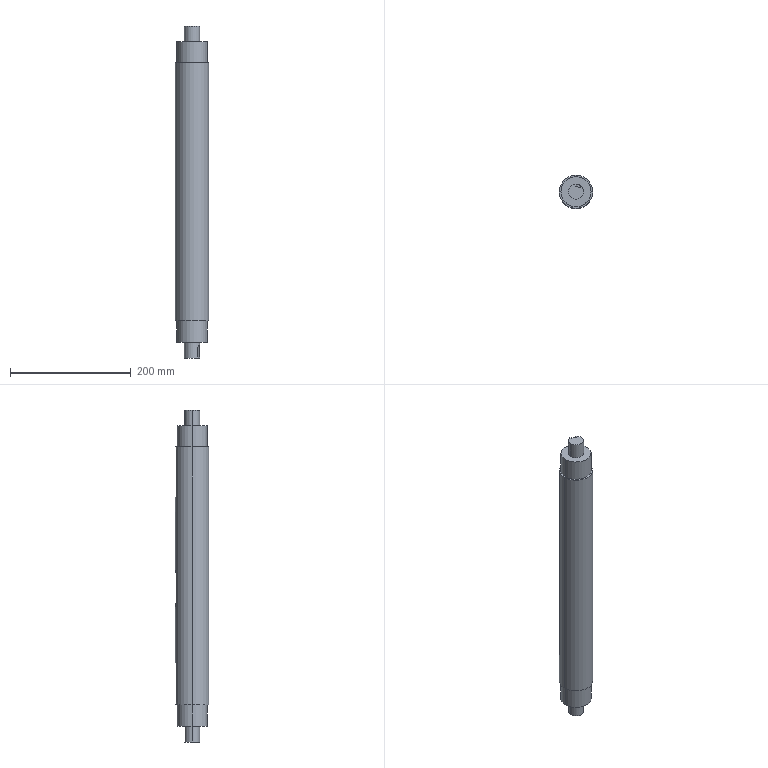Part | SolidWorks | features Cut 2, ICE 1, Revolution 1 | 1 solid | 30 faces | box 55 x 55 x 548.93 mm | volume 1170773 mm3 | cylinder 15 | plane 15 | commonest cylinder face diameters 25 x4 50 x4 16 x3 8 x2 55 x2
STEP:
#1=CARTESIAN_POINT('',(0.,21.5,183.93));
#2=VERTEX_POINT('',#1);
#3=CARTESIAN_POINT('',(8.,21.5,175.93));
#4=VERTEX_POINT('',#3);
#5=CARTESIAN_POINT('',(0.,21.5,175.93));
#6=DIRECTION('',(0.,1.,0.));
#7=DIRECTION('',(0.,0.,1.));
#8=AXIS2_PLACEMENT_3D('',#5,#6,#7);
#9=CIRCLE('',#8,8.);
#10=EDGE_CURVE('',#2,#4,#9,.T.);
#11=ORIENTED_EDGE('',*,*,#10,.F.);
#12=CARTESIAN_POINT('',(0.,27.5,183.93));
#13=VERTEX_POINT('',#12);
#14=CARTESIAN_POINT('',(0.,21.5,183.93));
#15=DIRECTION('',(0.,1.,0.));
#16=VECTOR('',#15,1000.);
#17=LINE('',#14,#16);
#18=EDGE_CURVE('',#2,#13,#17,.T.);
#19=ORIENTED_EDGE('',*,*,#18,.T.);
#20=CARTESIAN_POINT('',(8.,26.311,175.93));
#21=VERTEX_POINT('',#20);
#22=CARTESIAN_POINT('',(0.,27.5,183.93));
#23=CARTESIAN_POINT('',(0.5246,27.5,183.93));
#24=CARTESIAN_POINT('',(1.057,27.484,183.877));
#25=CARTESIAN_POINT('',(2.085,27.426,183.671));
#26=CARTESIAN_POINT('',(2.585,27.383,183.519));
#27=CARTESIAN_POINT('',(3.313,27.301,183.216));
#28=CARTESIAN_POINT('',(3.552,27.271,183.103));
#29=CARTESIAN_POINT('',(4.012,27.207,182.856));
#30=CARTESIAN_POINT('',(4.235,27.173,182.722));
#31=CARTESIAN_POINT('',(4.666,27.102,182.433));
#32=CARTESIAN_POINT('',(4.875,27.065,182.278));
#33=CARTESIAN_POINT('',(5.278,26.99,181.948));
#34=CARTESIAN_POINT('',(5.473,26.951,181.771));
#35=CARTESIAN_POINT('',(6.027,26.834,181.217));
#36=CARTESIAN_POINT('',(6.356,26.757,180.816));
#37=CARTESIAN_POINT('',(6.934,26.613,179.953));
#38=CARTESIAN_POINT('',(7.186,26.545,179.485));
#39=CARTESIAN_POINT('',(7.586,26.434,178.522));
#40=CARTESIAN_POINT('',(7.739,26.389,178.024));
#41=CARTESIAN_POINT('',(7.895,26.342,177.25));
#42=CARTESIAN_POINT('',(7.934,26.331,176.987));
#43=CARTESIAN_POINT('',(7.987,26.315,176.46));
#44=CARTESIAN_POINT('',(8.,26.311,176.196));
#45=CARTESIAN_POINT('',(8.,26.311,175.93));
#46=B_SPLINE_CURVE_WITH_KNOTS('',3,(#22,#23,#24,#25,#26,#27,#28,#29,#30,#31,#32,#33,#34,#35,#36,#37,#38,#39,#40,#41,#42,#43,#44,#45),.UNSPECIFIED.,.F.,.F.,(4,2,2,2,2,2,2,2,2,2,2,4),(0.01258,0.01415,0.01572,0.0165,0.01729,0.01807,0.01886,0.02043,0.022,0.02357,0.02435,0.02514),.UNSPECIFIED.);
#47=EDGE_CURVE('',#13,#21,#46,.T.);
#48=ORIENTED_EDGE('',*,*,#47,.T.);
#49=CARTESIAN_POINT('',(8.,21.5,175.93));
#50=DIRECTION('',(0.,1.,0.));
#51=VECTOR('',#50,1000.);
#52=LINE('',#49,#51);
#53=EDGE_CURVE('',#4,#21,#52,.T.);
#54=ORIENTED_EDGE('',*,*,#53,.F.);
#55=EDGE_LOOP('',(#11,#19,#48,#54));
#56=FACE_OUTER_BOUND('',#55,.T.);
#57=CARTESIAN_POINT('',(0.,21.5,175.93));
#58=DIRECTION('',(0.,1.,0.));
#59=DIRECTION('',(0.,0.,1.));
#60=AXIS2_PLACEMENT_3D('',#57,#58,#59);
#61=CYLINDRICAL_SURFACE('',#60,8.);
#62=ADVANCED_FACE('',(#56),#61,.F.);
#63=CARTESIAN_POINT('',(-25.,0.,422.93));
#64=VERTEX_POINT('',#63);
#65=CARTESIAN_POINT('',(25.,0.,422.93));
#66=VERTEX_POINT('',#65);
#67=CARTESIAN_POINT('',(0.,0.,422.93));
#68=DIRECTION('',(0.,0.,-1.));
#69=DIRECTION('',(-1.,0.,0.));
#70=AXIS2_PLACEMENT_3D('',#67,#68,#69);
#71=CIRCLE('',#70,25.);
#72=EDGE_CURVE('',#64,#66,#71,.T.);
#73=ORIENTED_EDGE('',*,*,#72,.T.);
#74=CARTESIAN_POINT('',(25.,0.,387.93));
#75=VERTEX_POINT('',#74);
#76=CARTESIAN_POINT('',(25.,0.,0.));
#77=DIRECTION('',(0.,0.,-1.));
#78=VECTOR('',#77,1000.);
#79=LINE('',#76,#78);
#80=EDGE_CURVE('',#66,#75,#79,.T.);
#81=ORIENTED_EDGE('',*,*,#80,.T.);
#82=CARTESIAN_POINT('',(-25.,0.,387.93));
#83=VERTEX_POINT('',#82);
#84=CARTESIAN_POINT('',(0.,0.,387.93));
#85=DIRECTION('',(0.,0.,-1.));
#86=DIRECTION('',(-1.,0.,0.));
#87=AXIS2_PLACEMENT_3D('',#84,#85,#86);
#88=CIRCLE('',#87,25.);
#89=EDGE_CURVE('',#83,#75,#88,.T.);
#90=ORIENTED_EDGE('',*,*,#89,.F.);
#91=CARTESIAN_POINT('',(-25.,0.,0.));
#92=DIRECTION('',(0.,0.,-1.));
#93=VECTOR('',#92,1000.);
#94=LINE('',#91,#93);
#95=EDGE_CURVE('',#64,#83,#94,.T.);
#96=ORIENTED_EDGE('',*,*,#95,.F.);
#97=EDGE_LOOP('',(#73,#81,#90,#96));
#98=FACE_OUTER_BOUND('',#97,.T.);
#99=CARTESIAN_POINT('',(0.,0.,0.));
#100=DIRECTION('',(0.,0.,-1.));
#101=DIRECTION('',(-1.,0.,0.));
#102=AXIS2_PLACEMENT_3D('',#99,#100,#101);
#103=CYLINDRICAL_SURFACE('',#102,25.);
#104=ADVANCED_FACE('',(#98),#103,.T.);
#105=CARTESIAN_POINT('',(-8.,26.311,175.93));
#106=VERTEX_POINT('',#105);
#107=CARTESIAN_POINT('',(-8.,26.311,175.93));
#108=CARTESIAN_POINT('',(-8.,26.311,176.462));
#109=CARTESIAN_POINT('',(-7.947,26.327,176.984));
#110=CARTESIAN_POINT('',(-7.794,26.373,177.754));
#111=CARTESIAN_POINT('',(-7.73,26.391,178.009));
#112=CARTESIAN_POINT('',(-7.576,26.436,178.513));
#113=CARTESIAN_POINT('',(-7.486,26.462,178.763));
#114=CARTESIAN_POINT('',(-7.184,26.546,179.488));
#115=CARTESIAN_POINT('',(-6.938,26.612,179.947));
#116=CARTESIAN_POINT('',(-6.503,26.721,180.597));
#117=CARTESIAN_POINT('',(-6.345,26.758,180.809));
#118=CARTESIAN_POINT('',(-6.013,26.835,181.213));
#119=CARTESIAN_POINT('',(-5.838,26.874,181.406));
#120=CARTESIAN_POINT('',(-5.287,26.99,181.956));
#121=CARTESIAN_POINT('',(-4.886,27.066,182.286));
#122=CARTESIAN_POINT('',(-4.012,27.209,182.871));
#123=CARTESIAN_POINT('',(-3.551,27.274,183.118));
#124=CARTESIAN_POINT('',(-2.829,27.355,183.418));
#125=CARTESIAN_POINT('',(-2.583,27.38,183.506));
#126=CARTESIAN_POINT('',(-2.081,27.422,183.659));
#127=CARTESIAN_POINT('',(-1.822,27.441,183.724));
#128=CARTESIAN_POINT('',(-1.047,27.485,183.879));
#129=CARTESIAN_POINT('',(-0.5252,27.5,183.93));
#130=CARTESIAN_POINT('',(0.,27.5,183.93));
#131=B_SPLINE_CURVE_WITH_KNOTS('',3,(#107,#108,#109,#110,#111,#112,#113,#114,#115,#116,#117,#118,#119,#120,#121,#122,#123,#124,#125,#126,#127,#128,#129,#130),.UNSPECIFIED.,.F.,.F.,(4,2,2,2,2,2,2,2,2,2,2,4),(0.,0.001572,0.002358,0.003144,0.004717,0.005503,0.006289,0.007861,0.009433,0.01022,0.01101,0.01258),.UNSPECIFIED.);
#132=EDGE_CURVE('',#106,#13,#131,.T.);
#133=ORIENTED_EDGE('',*,*,#132,.F.);
#134=CARTESIAN_POINT('',(-8.,26.311,131.93));
#135=VERTEX_POINT('',#134);
#136=CARTESIAN_POINT('',(-8.,26.311,0.));
#137=DIRECTION('',(0.,0.,1.));
#138=VECTOR('',#137,1000.);
#139=LINE('',#136,#138);
#140=EDGE_CURVE('',#135,#106,#139,.T.);
#141=ORIENTED_EDGE('',*,*,#140,.F.);
#142=CARTESIAN_POINT('',(8.,26.311,131.93));
#143=VERTEX_POINT('',#142);
#144=CARTESIAN_POINT('',(8.,26.311,131.93));
#145=CARTESIAN_POINT('',(8.,26.311,131.398));
#146=CARTESIAN_POINT('',(7.948,26.327,130.876));
#147=CARTESIAN_POINT('',(7.794,26.372,130.107));
#148=CARTESIAN_POINT('',(7.73,26.391,129.853));
#149=CARTESIAN_POINT('',(7.577,26.436,129.349));
#150=CARTESIAN_POINT('',(7.487,26.461,129.099));
#151=CARTESIAN_POINT('',(7.185,26.546,128.374));
#152=CARTESIAN_POINT('',(6.94,26.612,127.916));
#153=CARTESIAN_POINT('',(6.504,26.72,127.265));
#154=CARTESIAN_POINT('',(6.347,26.758,127.054));
#155=CARTESIAN_POINT('',(6.015,26.835,126.649));
#156=CARTESIAN_POINT('',(5.841,26.873,126.457));
#157=CARTESIAN_POINT('',(5.29,26.989,125.907));
#158=CARTESIAN_POINT('',(4.89,27.065,125.577));
#159=CARTESIAN_POINT('',(4.016,27.209,124.991));
#160=CARTESIAN_POINT('',(3.556,27.273,124.745));
#161=CARTESIAN_POINT('',(2.835,27.355,124.445));
#162=CARTESIAN_POINT('',(2.589,27.379,124.356));
#163=CARTESIAN_POINT('',(2.087,27.422,124.203));
#164=CARTESIAN_POINT('',(1.829,27.44,124.137));
#165=CARTESIAN_POINT('',(1.054,27.485,123.982));
#166=CARTESIAN_POINT('',(0.5326,27.5,123.931));
#167=CARTESIAN_POINT('',(-0.5171,27.5,123.929));
#168=CARTESIAN_POINT('',(-1.05,27.485,123.982));
#169=CARTESIAN_POINT('',(-2.079,27.426,124.187));
#170=CARTESIAN_POINT('',(-2.579,27.383,124.339));
#171=CARTESIAN_POINT('',(-3.308,27.301,124.641));
#172=CARTESIAN_POINT('',(-3.547,27.271,124.755));
#173=CARTESIAN_POINT('',(-4.008,27.207,125.001));
#174=CARTESIAN_POINT('',(-4.231,27.173,125.135));
#175=CARTESIAN_POINT('',(-4.663,27.103,125.424));
#176=CARTESIAN_POINT('',(-4.871,27.066,125.579));
#177=CARTESIAN_POINT('',(-5.275,26.99,125.91));
#178=CARTESIAN_POINT('',(-5.47,26.951,126.087));
#179=CARTESIAN_POINT('',(-6.024,26.835,126.641));
#180=CARTESIAN_POINT('',(-6.354,26.758,127.041));
#181=CARTESIAN_POINT('',(-6.933,26.613,127.905));
#182=CARTESIAN_POINT('',(-7.185,26.546,128.373));
#183=CARTESIAN_POINT('',(-7.586,26.434,129.336));
#184=CARTESIAN_POINT('',(-7.739,26.389,129.835));
#185=CARTESIAN_POINT('',(-7.895,26.343,130.609));
#186=CARTESIAN_POINT('',(-7.934,26.331,130.872));
#187=CARTESIAN_POINT('',(-7.987,26.315,131.4));
#188=CARTESIAN_POINT('',(-8.,26.311,131.664));
#189=CARTESIAN_POINT('',(-8.,26.311,131.93));
#190=B_SPLINE_CURVE_WITH_KNOTS('',3,(#144,#145,#146,#147,#148,#149,#150,#151,#152,#153,#154,#155,#156,#157,#158,#159,#160,#161,#162,#163,#164,#165,#166,#167,#168,#169,#170,#171,#172,#173,#174,#175,#176,#177,#178,#179,#180,#181,#182,#183,#184,#185,#186,#187,#188,#189),.UNSPECIFIED.,.F.,.F.,(4,2,2,2,2,2,2,2,2,2,2,2,2,2,2,2,2,2,2,2,2,2,4),(0.,0.001571,0.002357,0.003142,0.004714,0.005499,0.006285,0.007856,0.009427,0.01021,0.011,0.01257,0.01414,0.01571,0.0165,0.01728,0.01807,0.01885,0.02043,0.022,0.02357,0.02435,0.02514),.UNSPECIFIED.);
#191=EDGE_CURVE('',#143,#135,#190,.T.);
#192=ORIENTED_EDGE('',*,*,#191,.F.);
#193=CARTESIAN_POINT('',(8.,26.311,0.));
#194=DIRECTION('',(0.,0.,-1.));
#195=VECTOR('',#194,1000.);
#196=LINE('',#193,#195);
#197=EDGE_CURVE('',#21,#143,#196,.T.);
#198=ORIENTED_EDGE('',*,*,#197,.F.);
#199=ORIENTED_EDGE('',*,*,#47,.F.);
#200=EDGE_LOOP('',(#133,#141,#192,#198,#199));
#201=FACE_BOUND('',#200,.T.);
#202=CARTESIAN_POINT('',(-27.5,0.,387.93));
#203=VERTEX_POINT('',#202);
#204=CARTESIAN_POINT('',(27.5,0.,387.93));
#205=VERTEX_POINT('',#204);
#206=CARTESIAN_POINT('',(0.,0.,387.93));
#207=DIRECTION('',(0.,0.,-1.));
#208=DIRECTION('',(-1.,0.,0.));
#209=AXIS2_PLACEMENT_3D('',#206,#207,#208);
#210=CIRCLE('',#209,27.5);
#211=EDGE_CURVE('',#203,#205,#210,.T.);
#212=ORIENTED_EDGE('',*,*,#211,.T.);
#213=CARTESIAN_POINT('',(27.5,0.,-38.53));
#214=VERTEX_POINT('',#213);
#215=CARTESIAN_POINT('',(27.5,0.,0.));
#216=DIRECTION('',(0.,0.,-1.));
#217=VECTOR('',#216,1000.);
#218=LINE('',#215,#217);
#219=EDGE_CURVE('',#205,#214,#218,.T.);
#220=ORIENTED_EDGE('',*,*,#219,.T.);
#221=CARTESIAN_POINT('',(-27.5,0.,-38.53));
#222=VERTEX_POINT('',#221);
#223=CARTESIAN_POINT('',(0.,0.,-38.53));
#224=DIRECTION('',(0.,0.,-1.));
#225=DIRECTION('',(-1.,0.,0.));
#226=AXIS2_PLACEMENT_3D('',#223,#224,#225);
#227=CIRCLE('',#226,27.5);
#228=EDGE_CURVE('',#222,#214,#227,.T.);
#229=ORIENTED_EDGE('',*,*,#228,.F.);
#230=CARTESIAN_POINT('',(-27.5,0.,0.));
#231=DIRECTION('',(0.,0.,-1.));
#232=VECTOR('',#231,1000.);
#233=LINE('',#230,#232);
#234=EDGE_CURVE('',#203,#222,#233,.T.);
#235=ORIENTED_EDGE('',*,*,#234,.F.);
#236=EDGE_LOOP('',(#212,#220,#229,#235));
#237=FACE_OUTER_BOUND('',#236,.T.);
#238=CARTESIAN_POINT('',(0.,0.,0.));
#239=DIRECTION('',(0.,0.,-1.));
#240=DIRECTION('',(-1.,0.,0.));
#241=AXIS2_PLACEMENT_3D('',#238,#239,#240);
#242=CYLINDRICAL_SURFACE('',#241,27.5);
#243=ADVANCED_FACE('',(#201,#237),#242,.T.);
#244=CARTESIAN_POINT('',(-25.,0.,-38.53));
#245=VERTEX_POINT('',#244);
#246=CARTESIAN_POINT('',(25.,0.,-38.53));
#247=VERTEX_POINT('',#246);
#248=CARTESIAN_POINT('',(0.,0.,-38.53));
#249=DIRECTION('',(0.,0.,-1.));
#250=DIRECTION('',(-1.,0.,0.));
#251=AXIS2_PLACEMENT_3D('',#248,#249,#250);
#252=CIRCLE('',#251,25.);
#253=EDGE_CURVE('',#245,#247,#252,.T.);
#254=ORIENTED_EDGE('',*,*,#253,.T.);
#255=CARTESIAN_POINT('',(25.,0.,-74.));
#256=VERTEX_POINT('',#255);
#257=CARTESIAN_POINT('',(25.,0.,0.));
#258=DIRECTION('',(0.,0.,-1.));
#259=VECTOR('',#258,1000.);
#260=LINE('',#257,#259);
#261=EDGE_CURVE('',#247,#256,#260,.T.);
#262=ORIENTED_EDGE('',*,*,#261,.T.);
#263=CARTESIAN_POINT('',(-25.,0.,-74.));
#264=VERTEX_POINT('',#263);
#265=CARTESIAN_POINT('',(0.,0.,-74.));
#266=DIRECTION('',(0.,0.,-1.));
#267=DIRECTION('',(-1.,0.,0.));
#268=AXIS2_PLACEMENT_3D('',#265,#266,#267);
#269=CIRCLE('',#268,25.);
#270=EDGE_CURVE('',#264,#256,#269,.T.);
#271=ORIENTED_EDGE('',*,*,#270,.F.);
#272=CARTESIAN_POINT('',(-25.,0.,0.));
#273=DIRECTION('',(0.,0.,-1.));
#274=VECTOR('',#273,1000.);
#275=LINE('',#272,#274);
#276=EDGE_CURVE('',#245,#264,#275,.T.);
#277=ORIENTED_EDGE('',*,*,#276,.F.);
#278=EDGE_LOOP('',(#254,#262,#271,#277));
#279=FACE_OUTER_BOUND('',#278,.T.);
#280=CARTESIAN_POINT('',(0.,0.,0.));
#281=DIRECTION('',(0.,0.,-1.));
#282=DIRECTION('',(-1.,0.,0.));
#283=AXIS2_PLACEMENT_3D('',#280,#281,#282);
#284=CYLINDRICAL_SURFACE('',#283,25.);
#285=ADVANCED_FACE('',(#279),#284,.T.);
#286=CARTESIAN_POINT('',(-12.5,0.,-74.));
#287=VERTEX_POINT('',#286);
#288=CARTESIAN_POINT('',(12.5,0.,-74.));
#289=VERTEX_POINT('',#288);
#290=CARTESIAN_POINT('',(0.,0.,-74.));
#291=DIRECTION('',(0.,0.,-1.));
#292=DIRECTION('',(-1.,0.,0.));
#293=AXIS2_PLACEMENT_3D('',#290,#291,#292);
#294=CIRCLE('',#293,12.5);
#295=EDGE_CURVE('',#287,#289,#294,.T.);
#296=ORIENTED_EDGE('',*,*,#295,.T.);
#297=CARTESIAN_POINT('',(12.5,0.,-100.));
#298=VERTEX_POINT('',#297);
#299=CARTESIAN_POINT('',(12.5,0.,0.));
#300=DIRECTION('',(0.,0.,-1.));
#301=VECTOR('',#300,1000.);
#302=LINE('',#299,#301);
#303=EDGE_CURVE('',#289,#298,#302,.T.);
#304=ORIENTED_EDGE('',*,*,#303,.T.);
#305=CARTESIAN_POINT('',(-12.5,0.,-100.));
#306=VERTEX_POINT('',#305);
#307=CARTESIAN_POINT('',(0.,0.,-100.));
#308=DIRECTION('',(0.,0.,-1.));
#309=DIRECTION('',(-1.,0.,0.));
#310=AXIS2_PLACEMENT_3D('',#307,#308,#309);
#311=CIRCLE('',#310,12.5);
#312=EDGE_CURVE('',#306,#298,#311,.T.);
#313=ORIENTED_EDGE('',*,*,#312,.F.);
#314=CARTESIAN_POINT('',(-12.5,0.,0.));
#315=DIRECTION('',(0.,0.,-1.));
#316=VECTOR('',#315,1000.);
#317=LINE('',#314,#316);
#318=EDGE_CURVE('',#287,#306,#317,.T.);
#319=ORIENTED_EDGE('',*,*,#318,.F.);
#320=EDGE_LOOP('',(#296,#304,#313,#319));
#321=FACE_OUTER_BOUND('',#320,.T.);
#322=CARTESIAN_POINT('',(0.,0.,0.));
#323=DIRECTION('',(0.,0.,-1.));
#324=DIRECTION('',(-1.,0.,0.));
#325=AXIS2_PLACEMENT_3D('',#322,#323,#324);
#326=CYLINDRICAL_SURFACE('',#325,12.5);
#327=ADVANCED_FACE('',(#321),#326,.T.);
#328=CARTESIAN_POINT('',(8.471,9.192,448.93));
#329=VERTEX_POINT('',#328);
#330=CARTESIAN_POINT('',(12.5,0.,448.93));
#331=VERTEX_POINT('',#330);
#332=CARTESIAN_POINT('',(0.,0.,448.93));
#333=DIRECTION('',(0.,0.,-1.));
#334=DIRECTION('',(-1.,0.,0.));
#335=AXIS2_PLACEMENT_3D('',#332,#333,#334);
#336=CIRCLE('',#335,12.5);
#337=EDGE_CURVE('',#329,#331,#336,.T.);
#338=ORIENTED_EDGE('',*,*,#337,.T.);
#339=CARTESIAN_POINT('',(12.5,0.,422.93));
#340=VERTEX_POINT('',#339);
#341=CARTESIAN_POINT('',(12.5,0.,0.));
#342=DIRECTION('',(0.,0.,-1.));
#343=VECTOR('',#342,1000.);
#344=LINE('',#341,#343);
#345=EDGE_CURVE('',#331,#340,#344,.T.);
#346=ORIENTED_EDGE('',*,*,#345,.T.);
#347=CARTESIAN_POINT('',(-12.5,0.,422.93));
#348=VERTEX_POINT('',#347);
#349=CARTESIAN_POINT('',(0.,0.,422.93));
#350=DIRECTION('',(0.,0.,-1.));
#351=DIRECTION('',(-1.,0.,0.));
#352=AXIS2_PLACEMENT_3D('',#349,#350,#351);
#353=CIRCLE('',#352,12.5);
#354=EDGE_CURVE('',#348,#340,#353,.T.);
#355=ORIENTED_EDGE('',*,*,#354,.F.);
#356=CARTESIAN_POINT('',(-12.5,0.,448.93));
#357=VERTEX_POINT('',#356);
#358=CARTESIAN_POINT('',(-12.5,0.,0.));
#359=DIRECTION('',(0.,0.,-1.));
#360=VECTOR('',#359,1000.);
#361=LINE('',#358,#360);
#362=EDGE_CURVE('',#357,#348,#361,.T.);
#363=ORIENTED_EDGE('',*,*,#362,.F.);
#364=CARTESIAN_POINT('',(1.163,12.446,448.93));
#365=VERTEX_POINT('',#364);
#366=CARTESIAN_POINT('',(0.,0.,448.93));
#367=DIRECTION('',(0.,0.,-1.));
#368=DIRECTION('',(-1.,0.,0.));
#369=AXIS2_PLACEMENT_3D('',#366,#367,#368);
#370=CIRCLE('',#369,12.5);
#371=EDGE_CURVE('',#357,#365,#370,.T.);
#372=ORIENTED_EDGE('',*,*,#371,.T.);
#373=CARTESIAN_POINT('',(1.163,12.446,431.93));
#374=VERTEX_POINT('',#373);
#375=CARTESIAN_POINT('',(1.163,12.446,0.));
#376=DIRECTION('',(0.,0.,-1.));
#377=VECTOR('',#376,1000.);
#378=LINE('',#375,#377);
#379=EDGE_CURVE('',#365,#374,#378,.T.);
#380=ORIENTED_EDGE('',*,*,#379,.T.);
#381=CARTESIAN_POINT('',(8.471,9.192,431.93));
#382=VERTEX_POINT('',#381);
#383=CARTESIAN_POINT('',(1.163,12.446,431.93));
#384=CARTESIAN_POINT('',(1.163,12.446,431.664));
#385=CARTESIAN_POINT('',(1.19,12.443,431.403));
#386=CARTESIAN_POINT('',(1.298,12.433,430.889));
#387=CARTESIAN_POINT('',(1.379,12.424,430.634));
#388=CARTESIAN_POINT('',(1.588,12.399,430.151));
#389=CARTESIAN_POINT('',(1.715,12.383,429.922));
#390=CARTESIAN_POINT('',(2.013,12.338,429.489));
#391=CARTESIAN_POINT('',(2.184,12.309,429.285));
#392=CARTESIAN_POINT('',(2.553,12.238,428.919));
#393=CARTESIAN_POINT('',(2.753,12.195,428.754));
#394=CARTESIAN_POINT('',(3.184,12.09,428.461));
#395=CARTESIAN_POINT('',(3.408,12.029,428.338));
#396=CARTESIAN_POINT('',(3.871,11.888,428.138));
#397=CARTESIAN_POINT('',(4.113,11.807,428.06));
#398=CARTESIAN_POINT('',(4.599,11.626,427.956));
#399=CARTESIAN_POINT('',(4.84,11.528,427.93));
#400=CARTESIAN_POINT('',(5.321,11.314,427.93));
#401=CARTESIAN_POINT('',(5.561,11.198,427.956));
#402=CARTESIAN_POINT('',(6.018,10.959,428.059));
#403=CARTESIAN_POINT('',(6.237,10.836,428.135));
#404=CARTESIAN_POINT('',(6.657,10.583,428.337));
#405=CARTESIAN_POINT('',(6.854,10.456,428.461));
#406=CARTESIAN_POINT('',(7.216,10.209,428.75));
#407=CARTESIAN_POINT('',(7.385,10.087,428.917));
#408=CARTESIAN_POINT('',(7.687,9.859,429.285));
#409=CARTESIAN_POINT('',(7.819,9.753,429.485));
#410=CARTESIAN_POINT('',(8.052,9.563,429.917));
#411=CARTESIAN_POINT('',(8.151,9.477,430.15));
#412=CARTESIAN_POINT('',(8.309,9.339,430.632));
#413=CARTESIAN_POINT('',(8.369,9.285,430.881));
#414=CARTESIAN_POINT('',(8.45,9.211,431.398));
#415=CARTESIAN_POINT('',(8.471,9.192,431.664));
#416=CARTESIAN_POINT('',(8.471,9.192,431.93));
#417=B_SPLINE_CURVE_WITH_KNOTS('',3,(#383,#384,#385,#386,#387,#388,#389,#390,#391,#392,#393,#394,#395,#396,#397,#398,#399,#400,#401,#402,#403,#404,#405,#406,#407,#408,#409,#410,#411,#412,#413,#414,#415,#416),.UNSPECIFIED.,.F.,.F.,(4,2,2,2,2,2,2,2,2,2,2,2,2,2,2,2,4),(0.,0.0007865,0.001573,0.00236,0.003146,0.003933,0.004719,0.005506,0.006292,0.007079,0.007865,0.008652,0.009438,0.01022,0.01101,0.0118,0.01258),.UNSPECIFIED.);
#418=EDGE_CURVE('',#374,#382,#417,.T.);
#419=ORIENTED_EDGE('',*,*,#418,.T.);
#420=CARTESIAN_POINT('',(8.471,9.192,0.));
#421=DIRECTION('',(0.,0.,1.));
#422=VECTOR('',#421,1000.);
#423=LINE('',#420,#422);
#424=EDGE_CURVE('',#382,#329,#423,.T.);
#425=ORIENTED_EDGE('',*,*,#424,.T.);
#426=EDGE_LOOP('',(#338,#346,#355,#363,#372,#380,#419,#425));
#427=FACE_OUTER_BOUND('',#426,.T.);
#428=CARTESIAN_POINT('',(0.,0.,0.));
#429=DIRECTION('',(0.,0.,-1.));
#430=DIRECTION('',(-1.,0.,0.));
#431=AXIS2_PLACEMENT_3D('',#428,#429,#430);
#432=CYLINDRICAL_SURFACE('',#431,12.5);
#433=ADVANCED_FACE('',(#427),#432,.T.);
#434=ORIENTED_EDGE('',*,*,#345,.F.);
#435=CARTESIAN_POINT('',(0.,0.,448.93));
#436=DIRECTION('',(0.,0.,-1.));
#437=DIRECTION('',(-1.,0.,0.));
#438=AXIS2_PLACEMENT_3D('',#435,#436,#437);
#439=CIRCLE('',#438,12.5);
#440=EDGE_CURVE('',#331,#357,#439,.T.);
#441=ORIENTED_EDGE('',*,*,#440,.T.);
#442=ORIENTED_EDGE('',*,*,#362,.T.);
#443=CARTESIAN_POINT('',(0.,0.,422.93));
#444=DIRECTION('',(0.,0.,-1.));
#445=DIRECTION('',(-1.,0.,0.));
#446=AXIS2_PLACEMENT_3D('',#443,#444,#445);
#447=CIRCLE('',#446,12.5);
#448=EDGE_CURVE('',#340,#348,#447,.T.);
#449=ORIENTED_EDGE('',*,*,#448,.F.);
#450=EDGE_LOOP('',(#434,#441,#442,#449));
#451=FACE_OUTER_BOUND('',#450,.T.);
#452=CARTESIAN_POINT('',(0.,0.,0.));
#453=DIRECTION('',(0.,0.,-1.));
#454=DIRECTION('',(-1.,0.,0.));
#455=AXIS2_PLACEMENT_3D('',#452,#453,#454);
#456=CYLINDRICAL_SURFACE('',#455,12.5);
#457=ADVANCED_FACE('',(#451),#456,.T.);
#458=CARTESIAN_POINT('',(-0.1969,9.392,448.93));
#459=VERTEX_POINT('',#458);
#460=CARTESIAN_POINT('',(7.111,6.138,448.93));
#461=VERTEX_POINT('',#460);
#462=CARTESIAN_POINT('',(-6.975,12.41,448.93));
#463=DIRECTION('',(0.9135,-0.4067,0.));
#464=VECTOR('',#463,1000.);
#465=LINE('',#462,#464);
#466=EDGE_CURVE('',#459,#461,#465,.T.);
#467=ORIENTED_EDGE('',*,*,#466,.F.);
#468=CARTESIAN_POINT('',(-5.722,-3.018,448.93));
#469=DIRECTION('',(0.4067,0.9135,0.));
#470=VECTOR('',#469,1000.);
#471=LINE('',#468,#470);
#472=EDGE_CURVE('',#459,#365,#471,.T.);
#473=ORIENTED_EDGE('',*,*,#472,.T.);
#474=ORIENTED_EDGE('',*,*,#371,.F.);
#475=ORIENTED_EDGE('',*,*,#440,.F.);
#476=ORIENTED_EDGE('',*,*,#337,.F.);
#477=CARTESIAN_POINT('',(1.586,-6.272,448.93));
#478=DIRECTION('',(-0.4067,-0.9135,0.));
#479=VECTOR('',#478,1000.);
#480=LINE('',#477,#479);
#481=EDGE_CURVE('',#329,#461,#480,.T.);
#482=ORIENTED_EDGE('',*,*,#481,.T.);
#483=EDGE_LOOP('',(#467,#473,#474,#475,#476,#482));
#484=FACE_OUTER_BOUND('',#483,.T.);
#485=CARTESIAN_POINT('',(-12.5,0.,448.93));
#486=DIRECTION('',(0.,0.,1.));
#487=DIRECTION('',(1.,0.,0.));
#488=AXIS2_PLACEMENT_3D('',#485,#486,#487);
#489=PLANE('',#488);
#490=ADVANCED_FACE('',(#484),#489,.T.);
#491=CARTESIAN_POINT('',(6.138,-7.111,-100.));
#492=VERTEX_POINT('',#491);
#493=CARTESIAN_POINT('',(9.392,0.1969,-100.));
#494=VERTEX_POINT('',#493);
#495=CARTESIAN_POINT('',(7.765,-3.457,-100.));
#496=DIRECTION('',(0.4067,0.9135,0.));
#497=VECTOR('',#496,1000.);
#498=LINE('',#495,#497);
#499=EDGE_CURVE('',#492,#494,#498,.T.);
#500=ORIENTED_EDGE('',*,*,#499,.F.);
#501=CARTESIAN_POINT('',(9.192,-8.471,-100.));
#502=VERTEX_POINT('',#501);
#503=CARTESIAN_POINT('',(-1.627,-3.654,-100.));
#504=DIRECTION('',(0.9135,-0.4067,0.));
#505=VECTOR('',#504,1000.);
#506=LINE('',#503,#505);
#507=EDGE_CURVE('',#492,#502,#506,.T.);
#508=ORIENTED_EDGE('',*,*,#507,.T.);
#509=CARTESIAN_POINT('',(0.,0.,-100.));
#510=DIRECTION('',(0.,0.,-1.));
#511=DIRECTION('',(-1.,0.,0.));
#512=AXIS2_PLACEMENT_3D('',#509,#510,#511);
#513=CIRCLE('',#512,12.5);
#514=EDGE_CURVE('',#502,#306,#513,.T.);
#515=ORIENTED_EDGE('',*,*,#514,.T.);
#516=ORIENTED_EDGE('',*,*,#312,.T.);
#517=CARTESIAN_POINT('',(12.446,-1.163,-100.));
#518=VERTEX_POINT('',#517);
#519=CARTESIAN_POINT('',(0.,0.,-100.));
#520=DIRECTION('',(0.,0.,-1.));
#521=DIRECTION('',(-1.,0.,0.));
#522=AXIS2_PLACEMENT_3D('',#519,#520,#521);
#523=CIRCLE('',#522,12.5);
#524=EDGE_CURVE('',#298,#518,#523,.T.);
#525=ORIENTED_EDGE('',*,*,#524,.T.);
#526=CARTESIAN_POINT('',(1.627,3.654,-100.));
#527=DIRECTION('',(-0.9135,0.4067,0.));
#528=VECTOR('',#527,1000.);
#529=LINE('',#526,#528);
#530=EDGE_CURVE('',#518,#494,#529,.T.);
#531=ORIENTED_EDGE('',*,*,#530,.T.);
#532=EDGE_LOOP('',(#500,#508,#515,#516,#525,#531));
#533=FACE_OUTER_BOUND('',#532,.T.);
#534=CARTESIAN_POINT('',(0.,0.,-100.));
#535=DIRECTION('',(0.,0.,-1.));
#536=DIRECTION('',(-1.,0.,0.));
#537=AXIS2_PLACEMENT_3D('',#534,#535,#536);
#538=PLANE('',#537);
#539=ADVANCED_FACE('',(#533),#538,.T.);
#540=ORIENTED_EDGE('',*,*,#303,.F.);
#541=CARTESIAN_POINT('',(0.,0.,-74.));
#542=DIRECTION('',(0.,0.,-1.));
#543=DIRECTION('',(-1.,0.,0.));
#544=AXIS2_PLACEMENT_3D('',#541,#542,#543);
#545=CIRCLE('',#544,12.5);
#546=EDGE_CURVE('',#289,#287,#545,.T.);
#547=ORIENTED_EDGE('',*,*,#546,.T.);
#548=ORIENTED_EDGE('',*,*,#318,.T.);
#549=ORIENTED_EDGE('',*,*,#514,.F.);
#550=CARTESIAN_POINT('',(9.192,-8.471,-83.));
#551=VERTEX_POINT('',#550);
#552=CARTESIAN_POINT('',(9.192,-8.471,0.));
#553=DIRECTION('',(0.,0.,1.));
#554=VECTOR('',#553,1000.);
#555=LINE('',#552,#554);
#556=EDGE_CURVE('',#502,#551,#555,.T.);
#557=ORIENTED_EDGE('',*,*,#556,.T.);
#558=CARTESIAN_POINT('',(12.446,-1.163,-83.));
#559=VERTEX_POINT('',#558);
#560=CARTESIAN_POINT('',(9.192,-8.471,-83.));
#561=CARTESIAN_POINT('',(9.192,-8.471,-82.734));
#562=CARTESIAN_POINT('',(9.211,-8.451,-82.473));
#563=CARTESIAN_POINT('',(9.284,-8.371,-81.959));
#564=CARTESIAN_POINT('',(9.338,-8.31,-81.704));
#565=CARTESIAN_POINT('',(9.477,-8.152,-81.221));
#566=CARTESIAN_POINT('',(9.56,-8.054,-80.992));
#567=CARTESIAN_POINT('',(9.752,-7.822,-80.559));
#568=CARTESIAN_POINT('',(9.859,-7.686,-80.355));
#569=CARTESIAN_POINT('',(10.086,-7.386,-79.989));
#570=CARTESIAN_POINT('',(10.206,-7.221,-79.824));
#571=CARTESIAN_POINT('',(10.456,-6.854,-79.531));
#572=CARTESIAN_POINT('',(10.582,-6.659,-79.408));
#573=CARTESIAN_POINT('',(10.832,-6.244,-79.208));
#574=CARTESIAN_POINT('',(10.957,-6.022,-79.13));
#575=CARTESIAN_POINT('',(11.197,-5.563,-79.026));
#576=CARTESIAN_POINT('',(11.311,-5.328,-79.));
#577=CARTESIAN_POINT('',(11.525,-4.848,-79.));
#578=CARTESIAN_POINT('',(11.625,-4.601,-79.026));
#579=CARTESIAN_POINT('',(11.805,-4.117,-79.129));
#580=CARTESIAN_POINT('',(11.885,-3.879,-79.205));
#581=CARTESIAN_POINT('',(12.028,-3.41,-79.407));
#582=CARTESIAN_POINT('',(12.09,-3.184,-79.531));
#583=CARTESIAN_POINT('',(12.194,-2.758,-79.82));
#584=CARTESIAN_POINT('',(12.238,-2.555,-79.987));
#585=CARTESIAN_POINT('',(12.309,-2.183,-80.355));
#586=CARTESIAN_POINT('',(12.337,-2.016,-80.555));
#587=CARTESIAN_POINT('',(12.382,-1.719,-80.987));
#588=CARTESIAN_POINT('',(12.399,-1.589,-81.22));
#589=CARTESIAN_POINT('',(12.424,-1.38,-81.702));
#590=CARTESIAN_POINT('',(12.432,-1.3,-81.951));
#591=CARTESIAN_POINT('',(12.443,-1.191,-82.468));
#592=CARTESIAN_POINT('',(12.446,-1.163,-82.734));
#593=CARTESIAN_POINT('',(12.446,-1.163,-83.));
#594=B_SPLINE_CURVE_WITH_KNOTS('',3,(#560,#561,#562,#563,#564,#565,#566,#567,#568,#569,#570,#571,#572,#573,#574,#575,#576,#577,#578,#579,#580,#581,#582,#583,#584,#585,#586,#587,#588,#589,#590,#591,#592,#593),.UNSPECIFIED.,.F.,.F.,(4,2,2,2,2,2,2,2,2,2,2,2,2,2,2,2,4),(0.,0.0007865,0.001573,0.00236,0.003146,0.003933,0.004719,0.005506,0.006292,0.007079,0.007865,0.008652,0.009438,0.01022,0.01101,0.0118,0.01258),.UNSPECIFIED.);
#595=EDGE_CURVE('',#551,#559,#594,.T.);
#596=ORIENTED_EDGE('',*,*,#595,.T.);
#597=CARTESIAN_POINT('',(12.446,-1.163,0.));
#598=DIRECTION('',(0.,0.,-1.));
#599=VECTOR('',#598,1000.);
#600=LINE('',#597,#599);
#601=EDGE_CURVE('',#559,#518,#600,.T.);
#602=ORIENTED_EDGE('',*,*,#601,.T.);
#603=ORIENTED_EDGE('',*,*,#524,.F.);
#604=EDGE_LOOP('',(#540,#547,#548,#549,#557,#596,#602,#603));
#605=FACE_OUTER_BOUND('',#604,.T.);
#606=CARTESIAN_POINT('',(0.,0.,0.));
#607=DIRECTION('',(0.,0.,-1.));
#608=DIRECTION('',(-1.,0.,0.));
#609=AXIS2_PLACEMENT_3D('',#606,#607,#608);
#610=CYLINDRICAL_SURFACE('',#609,12.5);
#611=ADVANCED_FACE('',(#605),#610,.T.);
#612=ORIENTED_EDGE('',*,*,#270,.T.);
#613=CARTESIAN_POINT('',(0.,0.,-74.));
#614=DIRECTION('',(0.,0.,-1.));
#615=DIRECTION('',(-1.,0.,0.));
#616=AXIS2_PLACEMENT_3D('',#613,#614,#615);
#617=CIRCLE('',#616,25.);
#618=EDGE_CURVE('',#256,#264,#617,.T.);
#619=ORIENTED_EDGE('',*,*,#618,.T.);
#620=EDGE_LOOP('',(#612,#619));
#621=FACE_OUTER_BOUND('',#620,.T.);
#622=ORIENTED_EDGE('',*,*,#295,.F.);
#623=ORIENTED_EDGE('',*,*,#546,.F.);
#624=EDGE_LOOP('',(#622,#623));
#625=FACE_BOUND('',#624,.T.);
#626=CARTESIAN_POINT('',(-12.5,0.,-74.));
#627=DIRECTION('',(0.,0.,-1.));
#628=DIRECTION('',(-1.,0.,0.));
#629=AXIS2_PLACEMENT_3D('',#626,#627,#628);
#630=PLANE('',#629);
#631=ADVANCED_FACE('',(#621,#625),#630,.T.);
#632=ORIENTED_EDGE('',*,*,#261,.F.);
#633=CARTESIAN_POINT('',(0.,0.,-38.53));
#634=DIRECTION('',(0.,0.,-1.));
#635=DIRECTION('',(-1.,0.,0.));
#636=AXIS2_PLACEMENT_3D('',#633,#634,#635);
#637=CIRCLE('',#636,25.);
#638=EDGE_CURVE('',#247,#245,#637,.T.);
#639=ORIENTED_EDGE('',*,*,#638,.T.);
#640=ORIENTED_EDGE('',*,*,#276,.T.);
#641=ORIENTED_EDGE('',*,*,#618,.F.);
#642=EDGE_LOOP('',(#632,#639,#640,#641));
#643=FACE_OUTER_BOUND('',#642,.T.);
#644=CARTESIAN_POINT('',(0.,0.,0.));
#645=DIRECTION('',(0.,0.,-1.));
#646=DIRECTION('',(-1.,0.,0.));
#647=AXIS2_PLACEMENT_3D('',#644,#645,#646);
#648=CYLINDRICAL_SURFACE('',#647,25.);
#649=ADVANCED_FACE('',(#643),#648,.T.);
#650=ORIENTED_EDGE('',*,*,#228,.T.);
#651=CARTESIAN_POINT('',(0.,0.,-38.53));
#652=DIRECTION('',(0.,0.,-1.));
#653=DIRECTION('',(-1.,0.,0.));
#654=AXIS2_PLACEMENT_3D('',#651,#652,#653);
#655=CIRCLE('',#654,27.5);
#656=EDGE_CURVE('',#214,#222,#655,.T.);
#657=ORIENTED_EDGE('',*,*,#656,.T.);
#658=EDGE_LOOP('',(#650,#657));
#659=FACE_OUTER_BOUND('',#658,.T.);
#660=ORIENTED_EDGE('',*,*,#253,.F.);
#661=ORIENTED_EDGE('',*,*,#638,.F.);
#662=EDGE_LOOP('',(#660,#661));
#663=FACE_BOUND('',#662,.T.);
#664=CARTESIAN_POINT('',(-25.,0.,-38.53));
#665=DIRECTION('',(0.,0.,-1.));
#666=DIRECTION('',(-1.,0.,0.));
#667=AXIS2_PLACEMENT_3D('',#664,#665,#666);
#668=PLANE('',#667);
#669=ADVANCED_FACE('',(#659,#663),#668,.T.);
#670=ORIENTED_EDGE('',*,*,#219,.F.);
#671=CARTESIAN_POINT('',(0.,0.,387.93));
#672=DIRECTION('',(0.,0.,-1.));
#673=DIRECTION('',(-1.,0.,0.));
#674=AXIS2_PLACEMENT_3D('',#671,#672,#673);
#675=CIRCLE('',#674,27.5);
#676=EDGE_CURVE('',#205,#203,#675,.T.);
#677=ORIENTED_EDGE('',*,*,#676,.T.);
#678=ORIENTED_EDGE('',*,*,#234,.T.);
#679=ORIENTED_EDGE('',*,*,#656,.F.);
#680=EDGE_LOOP('',(#670,#677,#678,#679));
#681=FACE_OUTER_BOUND('',#680,.T.);
#682=CARTESIAN_POINT('',(0.,0.,0.));
#683=DIRECTION('',(0.,0.,-1.));
#684=DIRECTION('',(-1.,0.,0.));
#685=AXIS2_PLACEMENT_3D('',#682,#683,#684);
#686=CYLINDRICAL_SURFACE('',#685,27.5);
#687=ADVANCED_FACE('',(#681),#686,.T.);
#688=ORIENTED_EDGE('',*,*,#89,.T.);
#689=CARTESIAN_POINT('',(0.,0.,387.93));
#690=DIRECTION('',(0.,0.,-1.));
#691=DIRECTION('',(-1.,0.,0.));
#692=AXIS2_PLACEMENT_3D('',#689,#690,#691);
#693=CIRCLE('',#692,25.);
#694=EDGE_CURVE('',#75,#83,#693,.T.);
#695=ORIENTED_EDGE('',*,*,#694,.T.);
#696=EDGE_LOOP('',(#688,#695));
#697=FACE_BOUND('',#696,.T.);
#698=ORIENTED_EDGE('',*,*,#211,.F.);
#699=ORIENTED_EDGE('',*,*,#676,.F.);
#700=EDGE_LOOP('',(#698,#699));
#701=FACE_OUTER_BOUND('',#700,.T.);
#702=CARTESIAN_POINT('',(-27.5,0.,387.93));
#703=DIRECTION('',(0.,0.,1.));
#704=DIRECTION('',(1.,0.,0.));
#705=AXIS2_PLACEMENT_3D('',#702,#703,#704);
#706=PLANE('',#705);
#707=ADVANCED_FACE('',(#697,#701),#706,.T.);
#708=ORIENTED_EDGE('',*,*,#80,.F.);
#709=CARTESIAN_POINT('',(0.,0.,422.93));
#710=DIRECTION('',(0.,0.,-1.));
#711=DIRECTION('',(-1.,0.,0.));
#712=AXIS2_PLACEMENT_3D('',#709,#710,#711);
#713=CIRCLE('',#712,25.);
#714=EDGE_CURVE('',#66,#64,#713,.T.);
#715=ORIENTED_EDGE('',*,*,#714,.T.);
#716=ORIENTED_EDGE('',*,*,#95,.T.);
#717=ORIENTED_EDGE('',*,*,#694,.F.);
#718=EDGE_LOOP('',(#708,#715,#716,#717));
#719=FACE_OUTER_BOUND('',#718,.T.);
#720=CARTESIAN_POINT('',(0.,0.,0.));
#721=DIRECTION('',(0.,0.,-1.));
#722=DIRECTION('',(-1.,0.,0.));
#723=AXIS2_PLACEMENT_3D('',#720,#721,#722);
#724=CYLINDRICAL_SURFACE('',#723,25.);
#725=ADVANCED_FACE('',(#719),#724,.T.);
#726=ORIENTED_EDGE('',*,*,#354,.T.);
#727=ORIENTED_EDGE('',*,*,#448,.T.);
#728=EDGE_LOOP('',(#726,#727));
#729=FACE_BOUND('',#728,.T.);
#730=ORIENTED_EDGE('',*,*,#72,.F.);
#731=ORIENTED_EDGE('',*,*,#714,.F.);
#732=EDGE_LOOP('',(#730,#731));
#733=FACE_OUTER_BOUND('',#732,.T.);
#734=CARTESIAN_POINT('',(-25.,0.,422.93));
#735=DIRECTION('',(0.,0.,1.));
#736=DIRECTION('',(1.,0.,0.));
#737=AXIS2_PLACEMENT_3D('',#734,#735,#736);
#738=PLANE('',#737);
#739=ADVANCED_FACE('',(#729,#733),#738,.T.);
#740=CARTESIAN_POINT('',(8.,21.5,131.93));
#741=VERTEX_POINT('',#740);
#742=CARTESIAN_POINT('',(8.,21.5,131.93));
#743=DIRECTION('',(0.,1.,0.));
#744=VECTOR('',#743,1000.);
#745=LINE('',#742,#744);
#746=EDGE_CURVE('',#741,#143,#745,.T.);
#747=ORIENTED_EDGE('',*,*,#746,.T.);
#748=ORIENTED_EDGE('',*,*,#191,.T.);
#749=CARTESIAN_POINT('',(-8.,21.5,131.93));
#750=VERTEX_POINT('',#749);
#751=CARTESIAN_POINT('',(-8.,21.5,131.93));
#752=DIRECTION('',(0.,1.,0.));
#753=VECTOR('',#752,1000.);
#754=LINE('',#751,#753);
#755=EDGE_CURVE('',#750,#135,#754,.T.);
#756=ORIENTED_EDGE('',*,*,#755,.F.);
#757=CARTESIAN_POINT('',(0.,21.5,131.93));
#758=DIRECTION('',(0.,1.,0.));
#759=DIRECTION('',(0.,0.,1.));
#760=AXIS2_PLACEMENT_3D('',#757,#758,#759);
#761=CIRCLE('',#760,8.);
#762=EDGE_CURVE('',#741,#750,#761,.T.);
#763=ORIENTED_EDGE('',*,*,#762,.F.);
#764=EDGE_LOOP('',(#747,#748,#756,#763));
#765=FACE_OUTER_BOUND('',#764,.T.);
#766=CARTESIAN_POINT('',(0.,21.5,131.93));
#767=DIRECTION('',(0.,1.,0.));
#768=DIRECTION('',(0.,0.,1.));
#769=AXIS2_PLACEMENT_3D('',#766,#767,#768);
#770=CYLINDRICAL_SURFACE('',#769,8.);
#771=ADVANCED_FACE('',(#765),#770,.F.);
#772=ORIENTED_EDGE('',*,*,#197,.T.);
#773=ORIENTED_EDGE('',*,*,#746,.F.);
#774=CARTESIAN_POINT('',(8.,21.5,131.93));
#775=DIRECTION('',(0.,0.,-1.));
#776=VECTOR('',#775,1000.);
#777=LINE('',#774,#776);
#778=EDGE_CURVE('',#4,#741,#777,.T.);
#779=ORIENTED_EDGE('',*,*,#778,.F.);
#780=ORIENTED_EDGE('',*,*,#53,.T.);
#781=EDGE_LOOP('',(#772,#773,#779,#780));
#782=FACE_OUTER_BOUND('',#781,.T.);
#783=CARTESIAN_POINT('',(8.,21.5,131.93));
#784=DIRECTION('',(1.,0.,0.));
#785=DIRECTION('',(0.,0.,-1.));
#786=AXIS2_PLACEMENT_3D('',#783,#784,#785);
#787=PLANE('',#786);
#788=ADVANCED_FACE('',(#782),#787,.F.);
#789=ORIENTED_EDGE('',*,*,#18,.F.);
#790=CARTESIAN_POINT('',(-8.,21.5,175.93));
#791=VERTEX_POINT('',#790);
#792=CARTESIAN_POINT('',(0.,21.5,175.93));
#793=DIRECTION('',(0.,1.,0.));
#794=DIRECTION('',(0.,0.,1.));
#795=AXIS2_PLACEMENT_3D('',#792,#793,#794);
#796=CIRCLE('',#795,8.);
#797=EDGE_CURVE('',#791,#2,#796,.T.);
#798=ORIENTED_EDGE('',*,*,#797,.F.);
#799=CARTESIAN_POINT('',(-8.,21.5,175.93));
#800=DIRECTION('',(0.,1.,0.));
#801=VECTOR('',#800,1000.);
#802=LINE('',#799,#801);
#803=EDGE_CURVE('',#791,#106,#802,.T.);
#804=ORIENTED_EDGE('',*,*,#803,.T.);
#805=ORIENTED_EDGE('',*,*,#132,.T.);
#806=EDGE_LOOP('',(#789,#798,#804,#805));
#807=FACE_OUTER_BOUND('',#806,.T.);
#808=CARTESIAN_POINT('',(0.,21.5,175.93));
#809=DIRECTION('',(0.,1.,0.));
#810=DIRECTION('',(0.,0.,1.));
#811=AXIS2_PLACEMENT_3D('',#808,#809,#810);
#812=CYLINDRICAL_SURFACE('',#811,8.);
#813=ADVANCED_FACE('',(#807),#812,.F.);
#814=ORIENTED_EDGE('',*,*,#140,.T.);
#815=ORIENTED_EDGE('',*,*,#803,.F.);
#816=CARTESIAN_POINT('',(-8.,21.5,131.93));
#817=DIRECTION('',(0.,0.,1.));
#818=VECTOR('',#817,1000.);
#819=LINE('',#816,#818);
#820=EDGE_CURVE('',#750,#791,#819,.T.);
#821=ORIENTED_EDGE('',*,*,#820,.F.);
#822=ORIENTED_EDGE('',*,*,#755,.T.);
#823=EDGE_LOOP('',(#814,#815,#821,#822));
#824=FACE_OUTER_BOUND('',#823,.T.);
#825=CARTESIAN_POINT('',(-8.,21.5,131.93));
#826=DIRECTION('',(-1.,0.,0.));
#827=DIRECTION('',(0.,0.,1.));
#828=AXIS2_PLACEMENT_3D('',#825,#826,#827);
#829=PLANE('',#828);
#830=ADVANCED_FACE('',(#824),#829,.F.);
#831=ORIENTED_EDGE('',*,*,#762,.T.);
#832=ORIENTED_EDGE('',*,*,#820,.T.);
#833=ORIENTED_EDGE('',*,*,#797,.T.);
#834=ORIENTED_EDGE('',*,*,#10,.T.);
#835=ORIENTED_EDGE('',*,*,#778,.T.);
#836=EDGE_LOOP('',(#831,#832,#833,#834,#835));
#837=FACE_OUTER_BOUND('',#836,.T.);
#838=CARTESIAN_POINT('',(0.,21.5,131.93));
#839=DIRECTION('',(0.,1.,0.));
#840=DIRECTION('',(0.,0.,1.));
#841=AXIS2_PLACEMENT_3D('',#838,#839,#840);
#842=PLANE('',#841);
#843=ADVANCED_FACE('',(#837),#842,.T.);
#844=CARTESIAN_POINT('',(6.138,-7.111,-83.));
#845=VERTEX_POINT('',#844);
#846=CARTESIAN_POINT('',(6.138,-7.111,-105.848));
#847=DIRECTION('',(0.,0.,1.));
#848=VECTOR('',#847,1000.);
#849=LINE('',#846,#848);
#850=EDGE_CURVE('',#492,#845,#849,.T.);
#851=ORIENTED_EDGE('',*,*,#850,.T.);
#852=CARTESIAN_POINT('',(6.138,-7.111,-83.));
#853=DIRECTION('',(0.9135,-0.4067,0.));
#854=VECTOR('',#853,1000.);
#855=LINE('',#852,#854);
#856=EDGE_CURVE('',#845,#551,#855,.T.);
#857=ORIENTED_EDGE('',*,*,#856,.T.);
#858=ORIENTED_EDGE('',*,*,#556,.F.);
#859=ORIENTED_EDGE('',*,*,#507,.F.);
#860=EDGE_LOOP('',(#851,#857,#858,#859));
#861=FACE_OUTER_BOUND('',#860,.T.);
#862=CARTESIAN_POINT('',(6.138,-7.111,-105.848));
#863=DIRECTION('',(0.4067,0.9135,0.));
#864=DIRECTION('',(-0.9135,0.4067,0.));
#865=AXIS2_PLACEMENT_3D('',#862,#863,#864);
#866=PLANE('',#865);
#867=ADVANCED_FACE('',(#861),#866,.T.);
#868=ORIENTED_EDGE('',*,*,#856,.F.);
#869=CARTESIAN_POINT('',(9.392,0.1969,-83.));
#870=VERTEX_POINT('',#869);
#871=CARTESIAN_POINT('',(7.765,-3.457,-83.));
#872=DIRECTION('',(-0.9135,0.4067,0.));
#873=DIRECTION('',(-0.4067,-0.9135,0.));
#874=AXIS2_PLACEMENT_3D('',#871,#872,#873);
#875=CIRCLE('',#874,4.);
#876=EDGE_CURVE('',#845,#870,#875,.T.);
#877=ORIENTED_EDGE('',*,*,#876,.T.);
#878=CARTESIAN_POINT('',(9.392,0.1969,-83.));
#879=DIRECTION('',(0.9135,-0.4067,0.));
#880=VECTOR('',#879,1000.);
#881=LINE('',#878,#880);
#882=EDGE_CURVE('',#870,#559,#881,.T.);
#883=ORIENTED_EDGE('',*,*,#882,.T.);
#884=ORIENTED_EDGE('',*,*,#595,.F.);
#885=EDGE_LOOP('',(#868,#877,#883,#884));
#886=FACE_OUTER_BOUND('',#885,.T.);
#887=CARTESIAN_POINT('',(7.765,-3.457,-83.));
#888=DIRECTION('',(0.9135,-0.4067,0.));
#889=DIRECTION('',(0.4067,0.9135,0.));
#890=AXIS2_PLACEMENT_3D('',#887,#888,#889);
#891=CYLINDRICAL_SURFACE('',#890,4.);
#892=ADVANCED_FACE('',(#886),#891,.F.);
#893=ORIENTED_EDGE('',*,*,#601,.F.);
#894=ORIENTED_EDGE('',*,*,#882,.F.);
#895=CARTESIAN_POINT('',(9.392,0.1969,-105.848));
#896=DIRECTION('',(0.,0.,-1.));
#897=VECTOR('',#896,1000.);
#898=LINE('',#895,#897);
#899=EDGE_CURVE('',#870,#494,#898,.T.);
#900=ORIENTED_EDGE('',*,*,#899,.T.);
#901=ORIENTED_EDGE('',*,*,#530,.F.);
#902=EDGE_LOOP('',(#893,#894,#900,#901));
#903=FACE_OUTER_BOUND('',#902,.T.);
#904=CARTESIAN_POINT('',(9.392,0.1969,-105.848));
#905=DIRECTION('',(-0.4067,-0.9135,0.));
#906=DIRECTION('',(0.9135,-0.4067,0.));
#907=AXIS2_PLACEMENT_3D('',#904,#905,#906);
#908=PLANE('',#907);
#909=ADVANCED_FACE('',(#903),#908,.T.);
#910=ORIENTED_EDGE('',*,*,#499,.T.);
#911=ORIENTED_EDGE('',*,*,#899,.F.);
#912=ORIENTED_EDGE('',*,*,#876,.F.);
#913=ORIENTED_EDGE('',*,*,#850,.F.);
#914=EDGE_LOOP('',(#910,#911,#912,#913));
#915=FACE_OUTER_BOUND('',#914,.T.);
#916=CARTESIAN_POINT('',(7.765,-3.457,-105.848));
#917=DIRECTION('',(-0.9135,0.4067,0.));
#918=DIRECTION('',(-0.4067,-0.9135,0.));
#919=AXIS2_PLACEMENT_3D('',#916,#917,#918);
#920=PLANE('',#919);
#921=ADVANCED_FACE('',(#915),#920,.F.);
#922=ORIENTED_EDGE('',*,*,#472,.F.);
#923=CARTESIAN_POINT('',(-0.1969,9.392,431.93));
#924=VERTEX_POINT('',#923);
#925=CARTESIAN_POINT('',(-0.1969,9.392,455.304));
#926=DIRECTION('',(0.,0.,-1.));
#927=VECTOR('',#926,1000.);
#928=LINE('',#925,#927);
#929=EDGE_CURVE('',#459,#924,#928,.T.);
#930=ORIENTED_EDGE('',*,*,#929,.T.);
#931=CARTESIAN_POINT('',(-0.1969,9.392,431.93));
#932=DIRECTION('',(0.4067,0.9135,0.));
#933=VECTOR('',#932,1000.);
#934=LINE('',#931,#933);
#935=EDGE_CURVE('',#924,#374,#934,.T.);
#936=ORIENTED_EDGE('',*,*,#935,.T.);
#937=ORIENTED_EDGE('',*,*,#379,.F.);
#938=EDGE_LOOP('',(#922,#930,#936,#937));
#939=FACE_OUTER_BOUND('',#938,.T.);
#940=CARTESIAN_POINT('',(-0.1969,9.392,455.304));
#941=DIRECTION('',(0.9135,-0.4067,0.));
#942=DIRECTION('',(0.4067,0.9135,0.));
#943=AXIS2_PLACEMENT_3D('',#940,#941,#942);
#944=PLANE('',#943);
#945=ADVANCED_FACE('',(#939),#944,.T.);
#946=ORIENTED_EDGE('',*,*,#935,.F.);
#947=CARTESIAN_POINT('',(7.111,6.138,431.93));
#948=VERTEX_POINT('',#947);
#949=CARTESIAN_POINT('',(3.457,7.765,431.93));
#950=DIRECTION('',(-0.4067,-0.9135,0.));
#951=DIRECTION('',(0.9135,-0.4067,0.));
#952=AXIS2_PLACEMENT_3D('',#949,#950,#951);
#953=CIRCLE('',#952,4.);
#954=EDGE_CURVE('',#924,#948,#953,.T.);
#955=ORIENTED_EDGE('',*,*,#954,.T.);
#956=CARTESIAN_POINT('',(7.111,6.138,431.93));
#957=DIRECTION('',(0.4067,0.9135,0.));
#958=VECTOR('',#957,1000.);
#959=LINE('',#956,#958);
#960=EDGE_CURVE('',#948,#382,#959,.T.);
#961=ORIENTED_EDGE('',*,*,#960,.T.);
#962=ORIENTED_EDGE('',*,*,#418,.F.);
#963=EDGE_LOOP('',(#946,#955,#961,#962));
#964=FACE_OUTER_BOUND('',#963,.T.);
#965=CARTESIAN_POINT('',(3.457,7.765,431.93));
#966=DIRECTION('',(0.4067,0.9135,0.));
#967=DIRECTION('',(-0.9135,0.4067,0.));
#968=AXIS2_PLACEMENT_3D('',#965,#966,#967);
#969=CYLINDRICAL_SURFACE('',#968,4.);
#970=ADVANCED_FACE('',(#964),#969,.F.);
#971=ORIENTED_EDGE('',*,*,#960,.F.);
#972=CARTESIAN_POINT('',(7.111,6.138,455.304));
#973=DIRECTION('',(0.,0.,1.));
#974=VECTOR('',#973,1000.);
#975=LINE('',#972,#974);
#976=EDGE_CURVE('',#948,#461,#975,.T.);
#977=ORIENTED_EDGE('',*,*,#976,.T.);
#978=ORIENTED_EDGE('',*,*,#481,.F.);
#979=ORIENTED_EDGE('',*,*,#424,.F.);
#980=EDGE_LOOP('',(#971,#977,#978,#979));
#981=FACE_OUTER_BOUND('',#980,.T.);
#982=CARTESIAN_POINT('',(7.111,6.138,455.304));
#983=DIRECTION('',(-0.9135,0.4067,0.));
#984=DIRECTION('',(-0.4067,-0.9135,0.));
#985=AXIS2_PLACEMENT_3D('',#982,#983,#984);
#986=PLANE('',#985);
#987=ADVANCED_FACE('',(#981),#986,.T.);
#988=ORIENTED_EDGE('',*,*,#466,.T.);
#989=ORIENTED_EDGE('',*,*,#976,.F.);
#990=ORIENTED_EDGE('',*,*,#954,.F.);
#991=ORIENTED_EDGE('',*,*,#929,.F.);
#992=EDGE_LOOP('',(#988,#989,#990,#991));
#993=FACE_OUTER_BOUND('',#992,.T.);
#994=CARTESIAN_POINT('',(3.457,7.765,455.304));
#995=DIRECTION('',(-0.4067,-0.9135,0.));
#996=DIRECTION('',(0.9135,-0.4067,0.));
#997=AXIS2_PLACEMENT_3D('',#994,#995,#996);
#998=PLANE('',#997);
#999=ADVANCED_FACE('',(#993),#998,.F.);
#1000=CLOSED_SHELL('',(#62,#104,#243,#285,#327,#433,#457,#490,#539,#611,#631,#649,#669,#687,#707,#725,#739,#771,#788,#813,#830,#843,#867,#892,#909,#921,#945,#970,#987,#999));
#1001=MANIFOLD_SOLID_BREP('',#1000);
#1002=CARTESIAN_POINT('',(0.,0.,0.));
#1003=DIRECTION('',(0.,0.,1.));
#1004=DIRECTION('',(1.,0.,0.));
#1005=AXIS2_PLACEMENT_3D('',#1002,#1003,#1004);
#1006=(LENGTH_UNIT()NAMED_UNIT(*)SI_UNIT(.MILLI.,.METRE.));
#1007=UNCERTAINTY_MEASURE_WITH_UNIT(LENGTH_MEASURE(0.00001),#1006,'','');
#1008=(NAMED_UNIT(*)PLANE_ANGLE_UNIT()SI_UNIT($,.RADIAN.));
#1009=(NAMED_UNIT(*)SI_UNIT($,.STERADIAN.)SOLID_ANGLE_UNIT());
#1010=(GEOMETRIC_REPRESENTATION_CONTEXT(3)GLOBAL_UNCERTAINTY_ASSIGNED_CONTEXT((#1007))GLOBAL_UNIT_ASSIGNED_CONTEXT((#1006,#1008,#1009))REPRESENTATION_CONTEXT('',''));
#1011=ADVANCED_BREP_SHAPE_REPRESENTATION('',(#1001,#1005),#1010);